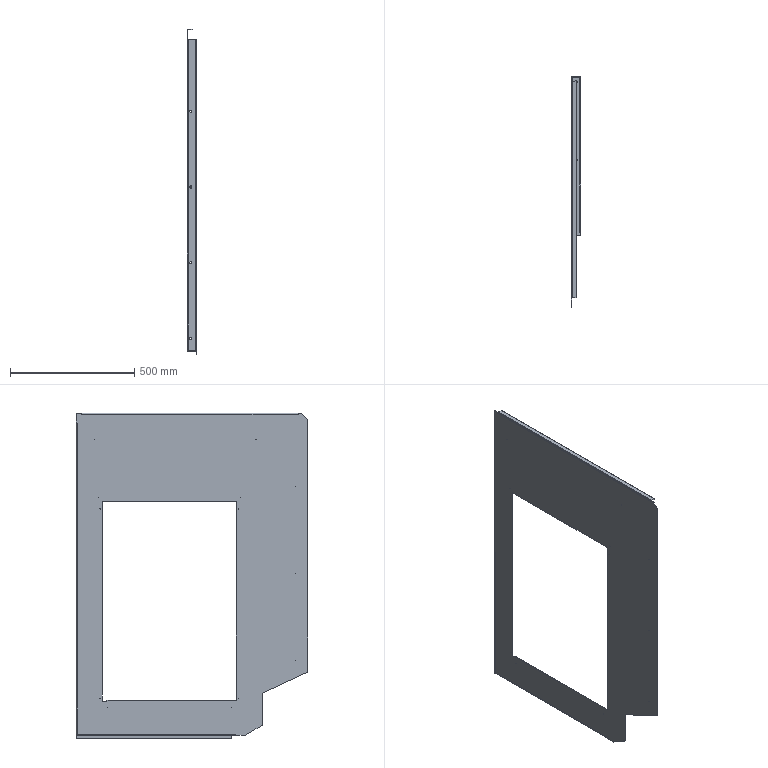Part | NX | features solid 2 | 1 solid | 101 faces | box 40 x 930 x 1310 mm | volume 1678188 mm3 | plane 53 | cylinder 48 | commonest cylinder face diameters 1 x26 9.2 x8 4 x5 8 x5 10 x4